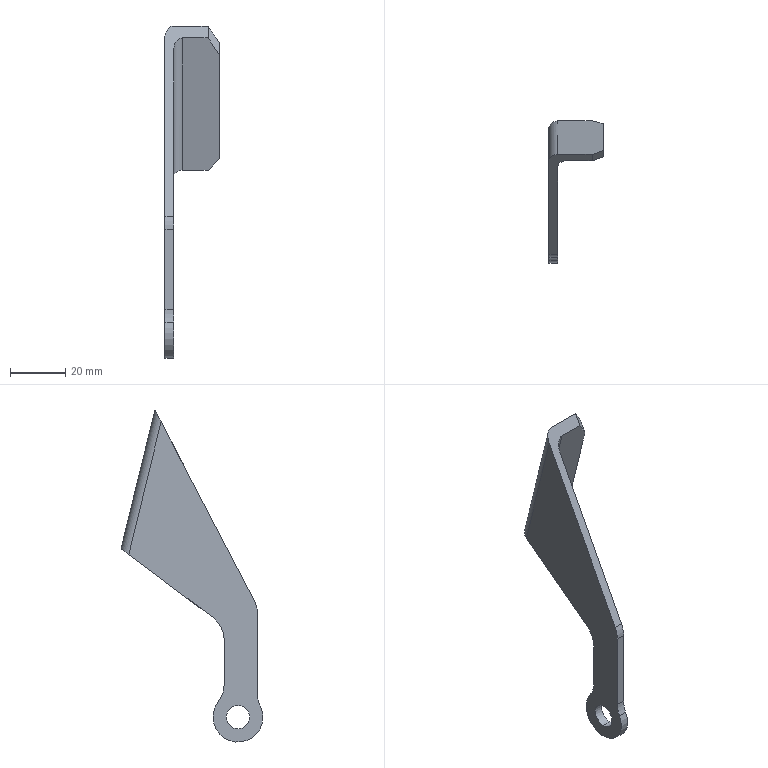Part | SolidWorks | features BaseBody 1 | 1 solid | 20 faces | box 19.6 x 51.2 x 119.9 mm | volume 9604 mm3 | plane 11 | cylinder 9 | commonest cylinder face diameters 20 x4 6.4 x2 8.479 x2 18 x1
STEP:
#1=CARTESIAN_POINT('',(1.6,0.,4.239));
#2=VERTEX_POINT('',#1);
#3=CARTESIAN_POINT('',(1.6,0.,-4.239));
#4=VERTEX_POINT('',#3);
#5=CARTESIAN_POINT('',(1.6,0.,0.));
#6=DIRECTION('',(1.,0.,0.));
#7=DIRECTION('',(0.,0.,1.));
#8=AXIS2_PLACEMENT_3D('',#5,#6,#7);
#9=CIRCLE('',#8,4.239);
#10=EDGE_CURVE('',#2,#4,#9,.T.);
#11=ORIENTED_EDGE('',*,*,#10,.T.);
#12=CARTESIAN_POINT('',(-1.6,0.,-4.239));
#13=VERTEX_POINT('',#12);
#14=CARTESIAN_POINT('',(1.6,0.,-4.239));
#15=DIRECTION('',(-1.,0.,0.));
#16=VECTOR('',#15,1000.);
#17=LINE('',#14,#16);
#18=EDGE_CURVE('',#4,#13,#17,.T.);
#19=ORIENTED_EDGE('',*,*,#18,.T.);
#20=CARTESIAN_POINT('',(-1.6,0.,4.239));
#21=VERTEX_POINT('',#20);
#22=CARTESIAN_POINT('',(-1.6,0.,0.));
#23=DIRECTION('',(-1.,0.,0.));
#24=DIRECTION('',(0.,0.,1.));
#25=AXIS2_PLACEMENT_3D('',#22,#23,#24);
#26=CIRCLE('',#25,4.239);
#27=EDGE_CURVE('',#13,#21,#26,.T.);
#28=ORIENTED_EDGE('',*,*,#27,.T.);
#29=CARTESIAN_POINT('',(1.6,0.,4.239));
#30=DIRECTION('',(-1.,0.,0.));
#31=VECTOR('',#30,1000.);
#32=LINE('',#29,#31);
#33=EDGE_CURVE('',#2,#21,#32,.T.);
#34=ORIENTED_EDGE('',*,*,#33,.F.);
#35=EDGE_LOOP('',(#11,#19,#28,#34));
#36=FACE_OUTER_BOUND('',#35,.T.);
#37=CARTESIAN_POINT('',(1.6,0.,0.));
#38=DIRECTION('',(-1.,0.,0.));
#39=DIRECTION('',(0.,0.,1.));
#40=AXIS2_PLACEMENT_3D('',#37,#38,#39);
#41=CYLINDRICAL_SURFACE('',#40,4.239);
#42=ADVANCED_FACE('',(#36),#41,.F.);
#43=ORIENTED_EDGE('',*,*,#18,.F.);
#44=CARTESIAN_POINT('',(1.6,0.,0.));
#45=DIRECTION('',(1.,0.,0.));
#46=DIRECTION('',(0.,0.,1.));
#47=AXIS2_PLACEMENT_3D('',#44,#45,#46);
#48=CIRCLE('',#47,4.239);
#49=EDGE_CURVE('',#4,#2,#48,.T.);
#50=ORIENTED_EDGE('',*,*,#49,.T.);
#51=ORIENTED_EDGE('',*,*,#33,.T.);
#52=CARTESIAN_POINT('',(-1.6,0.,0.));
#53=DIRECTION('',(-1.,0.,0.));
#54=DIRECTION('',(0.,0.,1.));
#55=AXIS2_PLACEMENT_3D('',#52,#53,#54);
#56=CIRCLE('',#55,4.239);
#57=EDGE_CURVE('',#21,#13,#56,.T.);
#58=ORIENTED_EDGE('',*,*,#57,.T.);
#59=EDGE_LOOP('',(#43,#50,#51,#58));
#60=FACE_OUTER_BOUND('',#59,.T.);
#61=CARTESIAN_POINT('',(1.6,0.,0.));
#62=DIRECTION('',(-1.,0.,0.));
#63=DIRECTION('',(0.,0.,1.));
#64=AXIS2_PLACEMENT_3D('',#61,#62,#63);
#65=CYLINDRICAL_SURFACE('',#64,4.239);
#66=ADVANCED_FACE('',(#60),#65,.F.);
#67=ORIENTED_EDGE('',*,*,#57,.F.);
#68=ORIENTED_EDGE('',*,*,#27,.F.);
#69=EDGE_LOOP('',(#67,#68));
#70=FACE_BOUND('',#69,.T.);
#71=CARTESIAN_POINT('',(-1.6,-7.,8.485));
#72=VERTEX_POINT('',#71);
#73=CARTESIAN_POINT('',(-1.6,-7.,37.451));
#74=VERTEX_POINT('',#73);
#75=CARTESIAN_POINT('',(-1.6,-7.,48.797));
#76=DIRECTION('',(0.,0.,1.));
#77=VECTOR('',#76,1000.);
#78=LINE('',#75,#77);
#79=EDGE_CURVE('',#72,#74,#78,.T.);
#80=ORIENTED_EDGE('',*,*,#79,.T.);
#81=CARTESIAN_POINT('',(-1.6,-5.868,42.072));
#82=VERTEX_POINT('',#81);
#83=CARTESIAN_POINT('',(-1.6,3.,37.451));
#84=DIRECTION('',(-1.,0.,0.));
#85=DIRECTION('',(0.,0.,1.));
#86=AXIS2_PLACEMENT_3D('',#83,#84,#85);
#87=CIRCLE('',#86,10.);
#88=EDGE_CURVE('',#74,#82,#87,.T.);
#89=ORIENTED_EDGE('',*,*,#88,.T.);
#90=CARTESIAN_POINT('',(-1.6,27.757,106.595));
#91=VERTEX_POINT('',#90);
#92=CARTESIAN_POINT('',(-1.6,-5.868,42.072));
#93=DIRECTION('',(0.,0.4621,0.8868));
#94=VECTOR('',#93,1000.);
#95=LINE('',#92,#94);
#96=EDGE_CURVE('',#82,#91,#95,.T.);
#97=ORIENTED_EDGE('',*,*,#96,.T.);
#98=CARTESIAN_POINT('',(-1.6,39.417,58.805));
#99=VERTEX_POINT('',#98);
#100=CARTESIAN_POINT('',(-1.6,27.757,106.595));
#101=DIRECTION('',(0.,0.237,-0.9715));
#102=VECTOR('',#101,1000.);
#103=LINE('',#100,#102);
#104=EDGE_CURVE('',#91,#99,#103,.T.);
#105=ORIENTED_EDGE('',*,*,#104,.T.);
#106=CARTESIAN_POINT('',(-1.6,8.986,35.9));
#107=VERTEX_POINT('',#106);
#108=CARTESIAN_POINT('',(-1.6,39.417,58.805));
#109=DIRECTION('',(0.,-0.799,-0.6014));
#110=VECTOR('',#109,1000.);
#111=LINE('',#108,#110);
#112=EDGE_CURVE('',#99,#107,#111,.T.);
#113=ORIENTED_EDGE('',*,*,#112,.T.);
#114=CARTESIAN_POINT('',(-1.6,5.,27.911));
#115=VERTEX_POINT('',#114);
#116=CARTESIAN_POINT('',(-1.6,15.,27.911));
#117=DIRECTION('',(1.,0.,0.));
#118=DIRECTION('',(0.,0.,1.));
#119=AXIS2_PLACEMENT_3D('',#116,#117,#118);
#120=CIRCLE('',#119,10.);
#121=EDGE_CURVE('',#107,#115,#120,.T.);
#122=ORIENTED_EDGE('',*,*,#121,.T.);
#123=CARTESIAN_POINT('',(-1.6,5.,11.662));
#124=VERTEX_POINT('',#123);
#125=CARTESIAN_POINT('',(-1.6,5.,48.797));
#126=DIRECTION('',(0.,0.,-1.));
#127=VECTOR('',#126,1000.);
#128=LINE('',#125,#127);
#129=EDGE_CURVE('',#115,#124,#128,.T.);
#130=ORIENTED_EDGE('',*,*,#129,.T.);
#131=CARTESIAN_POINT('',(-1.6,7.105,5.524));
#132=VERTEX_POINT('',#131);
#133=CARTESIAN_POINT('',(-1.6,15.,11.662));
#134=DIRECTION('',(1.,0.,0.));
#135=DIRECTION('',(0.,0.,1.));
#136=AXIS2_PLACEMENT_3D('',#133,#134,#135);
#137=CIRCLE('',#136,10.);
#138=EDGE_CURVE('',#124,#132,#137,.T.);
#139=ORIENTED_EDGE('',*,*,#138,.T.);
#140=CARTESIAN_POINT('',(-1.6,-8.053,4.019));
#141=VERTEX_POINT('',#140);
#142=CARTESIAN_POINT('',(-1.6,0.,0.));
#143=DIRECTION('',(-1.,0.,0.));
#144=DIRECTION('',(0.,0.,1.));
#145=AXIS2_PLACEMENT_3D('',#142,#143,#144);
#146=CIRCLE('',#145,9.);
#147=EDGE_CURVE('',#132,#141,#146,.T.);
#148=ORIENTED_EDGE('',*,*,#147,.T.);
#149=CARTESIAN_POINT('',(-1.6,-17.,8.485));
#150=DIRECTION('',(1.,0.,0.));
#151=DIRECTION('',(0.,0.,1.));
#152=AXIS2_PLACEMENT_3D('',#149,#150,#151);
#153=CIRCLE('',#152,10.);
#154=EDGE_CURVE('',#141,#72,#153,.T.);
#155=ORIENTED_EDGE('',*,*,#154,.T.);
#156=EDGE_LOOP('',(#80,#89,#97,#105,#113,#122,#130,#139,#148,#155));
#157=FACE_OUTER_BOUND('',#156,.T.);
#158=CARTESIAN_POINT('',(-1.6,-9.291,-9.694));
#159=DIRECTION('',(-1.,0.,0.));
#160=DIRECTION('',(0.,0.,1.));
#161=AXIS2_PLACEMENT_3D('',#158,#159,#160);
#162=PLANE('',#161);
#163=ADVANCED_FACE('',(#70,#157),#162,.T.);
#164=ORIENTED_EDGE('',*,*,#10,.F.);
#165=ORIENTED_EDGE('',*,*,#49,.F.);
#166=EDGE_LOOP('',(#164,#165));
#167=FACE_BOUND('',#166,.T.);
#168=CARTESIAN_POINT('',(1.6,25.513,102.29));
#169=VERTEX_POINT('',#168);
#170=CARTESIAN_POINT('',(1.6,36.634,56.711));
#171=VERTEX_POINT('',#170);
#172=CARTESIAN_POINT('',(1.6,36.706,56.416));
#173=DIRECTION('',(0.,0.237,-0.9715));
#174=VECTOR('',#173,1000.);
#175=LINE('',#172,#174);
#176=EDGE_CURVE('',#169,#171,#175,.T.);
#177=ORIENTED_EDGE('',*,*,#176,.F.);
#178=CARTESIAN_POINT('',(1.6,-5.868,42.072));
#179=VERTEX_POINT('',#178);
#180=CARTESIAN_POINT('',(1.6,-5.868,42.072));
#181=DIRECTION('',(0.,0.4621,0.8868));
#182=VECTOR('',#181,1000.);
#183=LINE('',#180,#182);
#184=EDGE_CURVE('',#179,#169,#183,.T.);
#185=ORIENTED_EDGE('',*,*,#184,.F.);
#186=CARTESIAN_POINT('',(1.6,-7.,37.451));
#187=VERTEX_POINT('',#186);
#188=CARTESIAN_POINT('',(1.6,3.,37.451));
#189=DIRECTION('',(-1.,0.,0.));
#190=DIRECTION('',(0.,0.,1.));
#191=AXIS2_PLACEMENT_3D('',#188,#189,#190);
#192=CIRCLE('',#191,10.);
#193=EDGE_CURVE('',#187,#179,#192,.T.);
#194=ORIENTED_EDGE('',*,*,#193,.F.);
#195=CARTESIAN_POINT('',(1.6,-7.,8.485));
#196=VERTEX_POINT('',#195);
#197=CARTESIAN_POINT('',(1.6,-7.,46.645));
#198=DIRECTION('',(0.,0.,1.));
#199=VECTOR('',#198,1000.);
#200=LINE('',#197,#199);
#201=EDGE_CURVE('',#196,#187,#200,.T.);
#202=ORIENTED_EDGE('',*,*,#201,.F.);
#203=CARTESIAN_POINT('',(1.6,-8.053,4.019));
#204=VERTEX_POINT('',#203);
#205=CARTESIAN_POINT('',(1.6,-17.,8.485));
#206=DIRECTION('',(1.,0.,0.));
#207=DIRECTION('',(0.,0.,1.));
#208=AXIS2_PLACEMENT_3D('',#205,#206,#207);
#209=CIRCLE('',#208,10.);
#210=EDGE_CURVE('',#204,#196,#209,.T.);
#211=ORIENTED_EDGE('',*,*,#210,.F.);
#212=CARTESIAN_POINT('',(1.6,7.105,5.524));
#213=VERTEX_POINT('',#212);
#214=CARTESIAN_POINT('',(1.6,0.,0.));
#215=DIRECTION('',(-1.,0.,0.));
#216=DIRECTION('',(0.,0.,1.));
#217=AXIS2_PLACEMENT_3D('',#214,#215,#216);
#218=CIRCLE('',#217,9.);
#219=EDGE_CURVE('',#213,#204,#218,.T.);
#220=ORIENTED_EDGE('',*,*,#219,.F.);
#221=CARTESIAN_POINT('',(1.6,5.,11.662));
#222=VERTEX_POINT('',#221);
#223=CARTESIAN_POINT('',(1.6,15.,11.662));
#224=DIRECTION('',(1.,0.,0.));
#225=DIRECTION('',(0.,0.,1.));
#226=AXIS2_PLACEMENT_3D('',#223,#224,#225);
#227=CIRCLE('',#226,10.);
#228=EDGE_CURVE('',#222,#213,#227,.T.);
#229=ORIENTED_EDGE('',*,*,#228,.F.);
#230=CARTESIAN_POINT('',(1.6,5.,27.911));
#231=VERTEX_POINT('',#230);
#232=CARTESIAN_POINT('',(1.6,5.,46.645));
#233=DIRECTION('',(0.,0.,-1.));
#234=VECTOR('',#233,1000.);
#235=LINE('',#232,#234);
#236=EDGE_CURVE('',#231,#222,#235,.T.);
#237=ORIENTED_EDGE('',*,*,#236,.F.);
#238=CARTESIAN_POINT('',(1.6,8.986,35.9));
#239=VERTEX_POINT('',#238);
#240=CARTESIAN_POINT('',(1.6,15.,27.911));
#241=DIRECTION('',(1.,0.,0.));
#242=DIRECTION('',(0.,0.,1.));
#243=AXIS2_PLACEMENT_3D('',#240,#241,#242);
#244=CIRCLE('',#243,10.);
#245=EDGE_CURVE('',#239,#231,#244,.T.);
#246=ORIENTED_EDGE('',*,*,#245,.F.);
#247=CARTESIAN_POINT('',(1.6,42.2,60.9));
#248=DIRECTION('',(0.,-0.799,-0.6014));
#249=VECTOR('',#248,1000.);
#250=LINE('',#247,#249);
#251=EDGE_CURVE('',#171,#239,#250,.T.);
#252=ORIENTED_EDGE('',*,*,#251,.F.);
#253=EDGE_LOOP('',(#177,#185,#194,#202,#211,#220,#229,#237,#246,#252));
#254=FACE_OUTER_BOUND('',#253,.T.);
#255=CARTESIAN_POINT('',(1.6,-9.274,-9.668));
#256=DIRECTION('',(-1.,0.,0.));
#257=DIRECTION('',(0.,0.,1.));
#258=AXIS2_PLACEMENT_3D('',#255,#256,#257);
#259=PLANE('',#258);
#260=ADVANCED_FACE('',(#167,#254),#259,.F.);
#261=CARTESIAN_POINT('',(0.,-7.,37.451));
#262=DIRECTION('',(-1.,0.,0.));
#263=VECTOR('',#262,1000.);
#264=LINE('',#261,#263);
#265=EDGE_CURVE('',#187,#74,#264,.T.);
#266=ORIENTED_EDGE('',*,*,#265,.F.);
#267=ORIENTED_EDGE('',*,*,#193,.T.);
#268=CARTESIAN_POINT('',(0.,-5.868,42.072));
#269=DIRECTION('',(1.,0.,0.));
#270=VECTOR('',#269,1000.);
#271=LINE('',#268,#270);
#272=EDGE_CURVE('',#82,#179,#271,.T.);
#273=ORIENTED_EDGE('',*,*,#272,.F.);
#274=ORIENTED_EDGE('',*,*,#88,.F.);
#275=EDGE_LOOP('',(#266,#267,#273,#274));
#276=FACE_OUTER_BOUND('',#275,.T.);
#277=CARTESIAN_POINT('',(1.6,3.,37.451));
#278=DIRECTION('',(-1.,0.,0.));
#279=DIRECTION('',(0.,0.,1.));
#280=AXIS2_PLACEMENT_3D('',#277,#278,#279);
#281=CYLINDRICAL_SURFACE('',#280,10.);
#282=ADVANCED_FACE('',(#276),#281,.T.);
#283=CARTESIAN_POINT('',(0.,-7.,8.485));
#284=DIRECTION('',(-1.,0.,0.));
#285=VECTOR('',#284,1000.);
#286=LINE('',#283,#285);
#287=EDGE_CURVE('',#196,#72,#286,.T.);
#288=ORIENTED_EDGE('',*,*,#287,.F.);
#289=ORIENTED_EDGE('',*,*,#201,.T.);
#290=ORIENTED_EDGE('',*,*,#265,.T.);
#291=ORIENTED_EDGE('',*,*,#79,.F.);
#292=EDGE_LOOP('',(#288,#289,#290,#291));
#293=FACE_OUTER_BOUND('',#292,.T.);
#294=CARTESIAN_POINT('',(-1.6,-7.,8.485));
#295=DIRECTION('',(0.,1.,0.));
#296=DIRECTION('',(0.,0.,1.));
#297=AXIS2_PLACEMENT_3D('',#294,#295,#296);
#298=PLANE('',#297);
#299=ADVANCED_FACE('',(#293),#298,.F.);
#300=ORIENTED_EDGE('',*,*,#210,.T.);
#301=ORIENTED_EDGE('',*,*,#287,.T.);
#302=ORIENTED_EDGE('',*,*,#154,.F.);
#303=CARTESIAN_POINT('',(0.,-8.053,4.019));
#304=DIRECTION('',(1.,0.,0.));
#305=VECTOR('',#304,1000.);
#306=LINE('',#303,#305);
#307=EDGE_CURVE('',#141,#204,#306,.T.);
#308=ORIENTED_EDGE('',*,*,#307,.T.);
#309=EDGE_LOOP('',(#300,#301,#302,#308));
#310=FACE_OUTER_BOUND('',#309,.T.);
#311=CARTESIAN_POINT('',(1.6,-17.,8.485));
#312=DIRECTION('',(-1.,0.,0.));
#313=DIRECTION('',(0.,0.,1.));
#314=AXIS2_PLACEMENT_3D('',#311,#312,#313);
#315=CYLINDRICAL_SURFACE('',#314,10.);
#316=ADVANCED_FACE('',(#310),#315,.F.);
#317=CARTESIAN_POINT('',(0.,7.105,5.524));
#318=DIRECTION('',(-1.,0.,0.));
#319=VECTOR('',#318,1000.);
#320=LINE('',#317,#319);
#321=EDGE_CURVE('',#213,#132,#320,.T.);
#322=ORIENTED_EDGE('',*,*,#321,.F.);
#323=ORIENTED_EDGE('',*,*,#219,.T.);
#324=ORIENTED_EDGE('',*,*,#307,.F.);
#325=ORIENTED_EDGE('',*,*,#147,.F.);
#326=EDGE_LOOP('',(#322,#323,#324,#325));
#327=FACE_OUTER_BOUND('',#326,.T.);
#328=CARTESIAN_POINT('',(1.6,0.,0.));
#329=DIRECTION('',(-1.,0.,0.));
#330=DIRECTION('',(0.,0.,1.));
#331=AXIS2_PLACEMENT_3D('',#328,#329,#330);
#332=CYLINDRICAL_SURFACE('',#331,9.);
#333=ADVANCED_FACE('',(#327),#332,.T.);
#334=ORIENTED_EDGE('',*,*,#228,.T.);
#335=ORIENTED_EDGE('',*,*,#321,.T.);
#336=ORIENTED_EDGE('',*,*,#138,.F.);
#337=CARTESIAN_POINT('',(0.,5.,11.662));
#338=DIRECTION('',(1.,0.,0.));
#339=VECTOR('',#338,1000.);
#340=LINE('',#337,#339);
#341=EDGE_CURVE('',#124,#222,#340,.T.);
#342=ORIENTED_EDGE('',*,*,#341,.T.);
#343=EDGE_LOOP('',(#334,#335,#336,#342));
#344=FACE_OUTER_BOUND('',#343,.T.);
#345=CARTESIAN_POINT('',(1.6,15.,11.662));
#346=DIRECTION('',(-1.,0.,0.));
#347=DIRECTION('',(0.,0.,1.));
#348=AXIS2_PLACEMENT_3D('',#345,#346,#347);
#349=CYLINDRICAL_SURFACE('',#348,10.);
#350=ADVANCED_FACE('',(#344),#349,.F.);
#351=CARTESIAN_POINT('',(0.,5.,27.911));
#352=DIRECTION('',(-1.,0.,0.));
#353=VECTOR('',#352,1000.);
#354=LINE('',#351,#353);
#355=EDGE_CURVE('',#231,#115,#354,.T.);
#356=ORIENTED_EDGE('',*,*,#355,.F.);
#357=ORIENTED_EDGE('',*,*,#236,.T.);
#358=ORIENTED_EDGE('',*,*,#341,.F.);
#359=ORIENTED_EDGE('',*,*,#129,.F.);
#360=EDGE_LOOP('',(#356,#357,#358,#359));
#361=FACE_OUTER_BOUND('',#360,.T.);
#362=CARTESIAN_POINT('',(-1.6,5.,27.911));
#363=DIRECTION('',(0.,-1.,0.));
#364=DIRECTION('',(0.,0.,-1.));
#365=AXIS2_PLACEMENT_3D('',#362,#363,#364);
#366=PLANE('',#365);
#367=ADVANCED_FACE('',(#361),#366,.F.);
#368=ORIENTED_EDGE('',*,*,#245,.T.);
#369=ORIENTED_EDGE('',*,*,#355,.T.);
#370=ORIENTED_EDGE('',*,*,#121,.F.);
#371=CARTESIAN_POINT('',(0.,8.986,35.9));
#372=DIRECTION('',(1.,0.,0.));
#373=VECTOR('',#372,1000.);
#374=LINE('',#371,#373);
#375=EDGE_CURVE('',#107,#239,#374,.T.);
#376=ORIENTED_EDGE('',*,*,#375,.T.);
#377=EDGE_LOOP('',(#368,#369,#370,#376));
#378=FACE_OUTER_BOUND('',#377,.T.);
#379=CARTESIAN_POINT('',(1.6,15.,27.911));
#380=DIRECTION('',(-1.,0.,0.));
#381=DIRECTION('',(0.,0.,1.));
#382=AXIS2_PLACEMENT_3D('',#379,#380,#381);
#383=CYLINDRICAL_SURFACE('',#382,10.);
#384=ADVANCED_FACE('',(#378),#383,.F.);
#385=CARTESIAN_POINT('',(1.6,42.2,60.9));
#386=VERTEX_POINT('',#385);
#387=CARTESIAN_POINT('',(1.6,42.2,60.9));
#388=CARTESIAN_POINT('',(-0.2745,42.2,60.9));
#389=CARTESIAN_POINT('',(-1.6,41.047,60.032));
#390=CARTESIAN_POINT('',(-1.6,39.417,58.805));
#391=(BOUNDED_CURVE()B_SPLINE_CURVE(3,(#387,#388,#389,#390),.UNSPECIFIED.,.F.,.F.)B_SPLINE_CURVE_WITH_KNOTS((4,4),(3.142,4.712),.UNSPECIFIED.)CURVE()GEOMETRIC_REPRESENTATION_ITEM()RATIONAL_B_SPLINE_CURVE((1.,0.8047,0.8047,1.))REPRESENTATION_ITEM(''));
#392=EDGE_CURVE('',#386,#99,#391,.T.);
#393=ORIENTED_EDGE('',*,*,#392,.F.);
#394=CARTESIAN_POINT('',(14.,42.2,60.9));
#395=VERTEX_POINT('',#394);
#396=CARTESIAN_POINT('',(6.2,42.2,60.9));
#397=DIRECTION('',(-1.,0.,0.));
#398=VECTOR('',#397,1000.);
#399=LINE('',#396,#398);
#400=EDGE_CURVE('',#395,#386,#399,.T.);
#401=ORIENTED_EDGE('',*,*,#400,.F.);
#402=CARTESIAN_POINT('',(14.,39.417,58.805));
#403=VERTEX_POINT('',#402);
#404=CARTESIAN_POINT('',(14.,25.593,48.4));
#405=DIRECTION('',(0.,0.799,0.6014));
#406=VECTOR('',#405,1000.);
#407=LINE('',#404,#406);
#408=EDGE_CURVE('',#403,#395,#407,.T.);
#409=ORIENTED_EDGE('',*,*,#408,.F.);
#410=CARTESIAN_POINT('',(4.8,39.417,58.805));
#411=VERTEX_POINT('',#410);
#412=CARTESIAN_POINT('',(6.2,39.417,58.805));
#413=DIRECTION('',(1.,0.,0.));
#414=VECTOR('',#413,1000.);
#415=LINE('',#412,#414);
#416=EDGE_CURVE('',#411,#403,#415,.T.);
#417=ORIENTED_EDGE('',*,*,#416,.F.);
#418=CARTESIAN_POINT('',(1.6,36.634,56.711));
#419=CARTESIAN_POINT('',(1.6,38.265,57.938));
#420=CARTESIAN_POINT('',(2.925,39.417,58.805));
#421=CARTESIAN_POINT('',(4.8,39.417,58.805));
#422=(BOUNDED_CURVE()B_SPLINE_CURVE(3,(#418,#419,#420,#421),.UNSPECIFIED.,.F.,.F.)B_SPLINE_CURVE_WITH_KNOTS((4,4),(4.712,6.283),.UNSPECIFIED.)CURVE()GEOMETRIC_REPRESENTATION_ITEM()RATIONAL_B_SPLINE_CURVE((1.,0.8047,0.8047,1.))REPRESENTATION_ITEM(''));
#423=EDGE_CURVE('',#171,#411,#422,.T.);
#424=ORIENTED_EDGE('',*,*,#423,.F.);
#425=ORIENTED_EDGE('',*,*,#251,.T.);
#426=ORIENTED_EDGE('',*,*,#375,.F.);
#427=ORIENTED_EDGE('',*,*,#112,.F.);
#428=EDGE_LOOP('',(#393,#401,#409,#417,#424,#425,#426,#427));
#429=FACE_OUTER_BOUND('',#428,.T.);
#430=CARTESIAN_POINT('',(-1.6,42.2,60.9));
#431=DIRECTION('',(0.,-0.6014,0.799));
#432=DIRECTION('',(0.,-0.799,-0.6014));
#433=AXIS2_PLACEMENT_3D('',#430,#431,#432);
#434=PLANE('',#433);
#435=ADVANCED_FACE('',(#429),#434,.F.);
#436=ORIENTED_EDGE('',*,*,#104,.F.);
#437=CARTESIAN_POINT('',(1.6,30.,110.9));
#438=VERTEX_POINT('',#437);
#439=CARTESIAN_POINT('',(1.6,30.,110.9));
#440=CARTESIAN_POINT('',(-0.2745,30.,110.9));
#441=CARTESIAN_POINT('',(-1.6,29.071,109.117));
#442=CARTESIAN_POINT('',(-1.6,27.757,106.595));
#443=(BOUNDED_CURVE()B_SPLINE_CURVE(3,(#439,#440,#441,#442),.UNSPECIFIED.,.F.,.F.)B_SPLINE_CURVE_WITH_KNOTS((4,4),(3.142,4.712),.UNSPECIFIED.)CURVE()GEOMETRIC_REPRESENTATION_ITEM()RATIONAL_B_SPLINE_CURVE((1.,0.8047,0.8047,1.))REPRESENTATION_ITEM(''));
#444=EDGE_CURVE('',#438,#91,#443,.T.);
#445=ORIENTED_EDGE('',*,*,#444,.F.);
#446=CARTESIAN_POINT('',(1.6,36.263,85.232));
#447=DIRECTION('',(0.,-0.237,0.9715));
#448=VECTOR('',#447,1000.);
#449=LINE('',#446,#448);
#450=EDGE_CURVE('',#386,#438,#449,.T.);
#451=ORIENTED_EDGE('',*,*,#450,.F.);
#452=ORIENTED_EDGE('',*,*,#392,.T.);
#453=EDGE_LOOP('',(#436,#445,#451,#452));
#454=FACE_OUTER_BOUND('',#453,.T.);
#455=CARTESIAN_POINT('',(1.6,26.816,110.449));
#456=DIRECTION('',(0.,0.237,-0.9715));
#457=DIRECTION('',(0.,0.9715,0.237));
#458=AXIS2_PLACEMENT_3D('',#455,#456,#457);
#459=CYLINDRICAL_SURFACE('',#458,3.2);
#460=ADVANCED_FACE('',(#454),#459,.T.);
#461=ORIENTED_EDGE('',*,*,#444,.T.);
#462=ORIENTED_EDGE('',*,*,#96,.F.);
#463=ORIENTED_EDGE('',*,*,#272,.T.);
#464=ORIENTED_EDGE('',*,*,#184,.T.);
#465=CARTESIAN_POINT('',(4.8,27.757,106.595));
#466=VERTEX_POINT('',#465);
#467=CARTESIAN_POINT('',(4.8,27.757,106.595));
#468=CARTESIAN_POINT('',(2.925,27.757,106.595));
#469=CARTESIAN_POINT('',(1.6,26.827,104.812));
#470=CARTESIAN_POINT('',(1.6,25.513,102.29));
#471=(BOUNDED_CURVE()B_SPLINE_CURVE(3,(#467,#468,#469,#470),.UNSPECIFIED.,.F.,.F.)B_SPLINE_CURVE_WITH_KNOTS((4,4),(0.,1.571),.UNSPECIFIED.)CURVE()GEOMETRIC_REPRESENTATION_ITEM()RATIONAL_B_SPLINE_CURVE((1.,0.8047,0.8047,1.))REPRESENTATION_ITEM(''));
#472=EDGE_CURVE('',#466,#169,#471,.T.);
#473=ORIENTED_EDGE('',*,*,#472,.F.);
#474=CARTESIAN_POINT('',(14.,27.757,106.595));
#475=VERTEX_POINT('',#474);
#476=CARTESIAN_POINT('',(6.2,27.757,106.595));
#477=DIRECTION('',(-1.,0.,0.));
#478=VECTOR('',#477,1000.);
#479=LINE('',#476,#478);
#480=EDGE_CURVE('',#475,#466,#479,.T.);
#481=ORIENTED_EDGE('',*,*,#480,.F.);
#482=CARTESIAN_POINT('',(14.,30.,110.9));
#483=VERTEX_POINT('',#482);
#484=CARTESIAN_POINT('',(14.,12.066,76.486));
#485=DIRECTION('',(0.,-0.4621,-0.8868));
#486=VECTOR('',#485,1000.);
#487=LINE('',#484,#486);
#488=EDGE_CURVE('',#483,#475,#487,.T.);
#489=ORIENTED_EDGE('',*,*,#488,.F.);
#490=CARTESIAN_POINT('',(6.2,30.,110.9));
#491=DIRECTION('',(1.,0.,0.));
#492=VECTOR('',#491,1000.);
#493=LINE('',#490,#492);
#494=EDGE_CURVE('',#438,#483,#493,.T.);
#495=ORIENTED_EDGE('',*,*,#494,.F.);
#496=EDGE_LOOP('',(#461,#462,#463,#464,#473,#481,#489,#495));
#497=FACE_OUTER_BOUND('',#496,.T.);
#498=CARTESIAN_POINT('',(-1.6,-5.868,42.072));
#499=DIRECTION('',(0.,0.8868,-0.4621));
#500=DIRECTION('',(0.,0.4621,0.8868));
#501=AXIS2_PLACEMENT_3D('',#498,#499,#500);
#502=PLANE('',#501);
#503=ADVANCED_FACE('',(#497),#502,.F.);
#504=ORIENTED_EDGE('',*,*,#472,.T.);
#505=ORIENTED_EDGE('',*,*,#176,.T.);
#506=ORIENTED_EDGE('',*,*,#423,.T.);
#507=CARTESIAN_POINT('',(4.8,33.75,82.032));
#508=DIRECTION('',(0.,-0.237,0.9715));
#509=VECTOR('',#508,1000.);
#510=LINE('',#507,#509);
#511=EDGE_CURVE('',#411,#466,#510,.T.);
#512=ORIENTED_EDGE('',*,*,#511,.T.);
#513=EDGE_LOOP('',(#504,#505,#506,#512));
#514=FACE_OUTER_BOUND('',#513,.T.);
#515=CARTESIAN_POINT('',(4.8,36.706,56.416));
#516=DIRECTION('',(0.,-0.237,0.9715));
#517=DIRECTION('',(0.,-0.9715,-0.237));
#518=AXIS2_PLACEMENT_3D('',#515,#516,#517);
#519=CYLINDRICAL_SURFACE('',#518,3.2);
#520=ADVANCED_FACE('',(#514),#519,.F.);
#521=ORIENTED_EDGE('',*,*,#450,.T.);
#522=ORIENTED_EDGE('',*,*,#494,.T.);
#523=CARTESIAN_POINT('',(18.,31.438,105.005));
#524=VERTEX_POINT('',#523);
#525=CARTESIAN_POINT('',(18.,31.438,105.005));
#526=DIRECTION('',(-0.5504,-0.1979,0.8111));
#527=VECTOR('',#526,1000.);
#528=LINE('',#525,#527);
#529=EDGE_CURVE('',#524,#483,#528,.T.);
#530=ORIENTED_EDGE('',*,*,#529,.F.);
#531=CARTESIAN_POINT('',(18.,41.168,65.13));
#532=VERTEX_POINT('',#531);
#533=CARTESIAN_POINT('',(18.,36.1,85.9));
#534=DIRECTION('',(0.,-0.237,0.9715));
#535=VECTOR('',#534,1000.);
#536=LINE('',#533,#535);
#537=EDGE_CURVE('',#532,#524,#536,.T.);
#538=ORIENTED_EDGE('',*,*,#537,.F.);
#539=CARTESIAN_POINT('',(14.,42.2,60.9));
#540=DIRECTION('',(0.6766,-0.1746,0.7154));
#541=VECTOR('',#540,1000.);
#542=LINE('',#539,#541);
#543=EDGE_CURVE('',#395,#532,#542,.T.);
#544=ORIENTED_EDGE('',*,*,#543,.F.);
#545=ORIENTED_EDGE('',*,*,#400,.T.);
#546=EDGE_LOOP('',(#521,#522,#530,#538,#544,#545));
#547=FACE_OUTER_BOUND('',#546,.T.);
#548=CARTESIAN_POINT('',(1.6,30.,110.9));
#549=DIRECTION('',(0.,-0.9715,-0.237));
#550=DIRECTION('',(0.,0.237,-0.9715));
#551=AXIS2_PLACEMENT_3D('',#548,#549,#550);
#552=PLANE('',#551);
#553=ADVANCED_FACE('',(#547),#552,.F.);
#554=CARTESIAN_POINT('',(18.,38.385,63.035));
#555=VERTEX_POINT('',#554);
#556=CARTESIAN_POINT('',(18.,38.385,63.035));
#557=DIRECTION('',(-0.6766,0.1746,-0.7154));
#558=VECTOR('',#557,1000.);
#559=LINE('',#556,#558);
#560=EDGE_CURVE('',#555,#403,#559,.T.);
#561=ORIENTED_EDGE('',*,*,#560,.T.);
#562=ORIENTED_EDGE('',*,*,#408,.T.);
#563=ORIENTED_EDGE('',*,*,#543,.T.);
#564=CARTESIAN_POINT('',(18.,41.168,65.13));
#565=DIRECTION('',(0.000000001,-0.799,-0.6014));
#566=VECTOR('',#565,1000.);
#567=LINE('',#564,#566);
#568=EDGE_CURVE('',#532,#555,#567,.T.);
#569=ORIENTED_EDGE('',*,*,#568,.T.);
#570=EDGE_LOOP('',(#561,#562,#563,#569));
#571=FACE_OUTER_BOUND('',#570,.T.);
#572=CARTESIAN_POINT('',(19.058,38.362,64.342));
#573=DIRECTION('',(0.7071,0.4252,-0.565));
#574=DIRECTION('',(-0.6242,0.,-0.7813));
#575=AXIS2_PLACEMENT_3D('',#572,#573,#574);
#576=PLANE('',#575);
#577=ADVANCED_FACE('',(#571),#576,.T.);
#578=CARTESIAN_POINT('',(18.,29.195,100.7));
#579=VERTEX_POINT('',#578);
#580=CARTESIAN_POINT('',(18.,33.587,82.7));
#581=DIRECTION('',(0.,-0.237,0.9715));
#582=VECTOR('',#581,1000.);
#583=LINE('',#580,#582);
#584=EDGE_CURVE('',#555,#579,#583,.T.);
#585=ORIENTED_EDGE('',*,*,#584,.T.);
#586=CARTESIAN_POINT('',(18.,29.195,100.7));
#587=DIRECTION('',(-0.5504,-0.1979,0.8111));
#588=VECTOR('',#587,1000.);
#589=LINE('',#586,#588);
#590=EDGE_CURVE('',#579,#475,#589,.T.);
#591=ORIENTED_EDGE('',*,*,#590,.T.);
#592=ORIENTED_EDGE('',*,*,#480,.T.);
#593=ORIENTED_EDGE('',*,*,#511,.F.);
#594=ORIENTED_EDGE('',*,*,#416,.T.);
#595=ORIENTED_EDGE('',*,*,#560,.F.);
#596=EDGE_LOOP('',(#585,#591,#592,#593,#594,#595));
#597=FACE_OUTER_BOUND('',#596,.T.);
#598=CARTESIAN_POINT('',(4.8,27.757,106.595));
#599=DIRECTION('',(0.,-0.9715,-0.237));
#600=DIRECTION('',(0.,0.237,-0.9715));
#601=AXIS2_PLACEMENT_3D('',#598,#599,#600);
#602=PLANE('',#601);
#603=ADVANCED_FACE('',(#597),#602,.T.);
#604=ORIENTED_EDGE('',*,*,#529,.T.);
#605=ORIENTED_EDGE('',*,*,#488,.T.);
#606=ORIENTED_EDGE('',*,*,#590,.F.);
#607=CARTESIAN_POINT('',(18.,29.195,100.7));
#608=DIRECTION('',(0.,0.4621,0.8868));
#609=VECTOR('',#608,1000.);
#610=LINE('',#607,#609);
#611=EDGE_CURVE('',#579,#524,#610,.T.);
#612=ORIENTED_EDGE('',*,*,#611,.T.);
#613=EDGE_LOOP('',(#604,#605,#606,#612));
#614=FACE_OUTER_BOUND('',#613,.T.);
#615=CARTESIAN_POINT('',(15.519,26.366,100.639));
#616=DIRECTION('',(0.7071,-0.6271,0.3268));
#617=DIRECTION('',(0.6635,0.7482,0.));
#618=AXIS2_PLACEMENT_3D('',#615,#616,#617);
#619=PLANE('',#618);
#620=ADVANCED_FACE('',(#614),#619,.T.);
#621=ORIENTED_EDGE('',*,*,#537,.T.);
#622=ORIENTED_EDGE('',*,*,#611,.F.);
#623=ORIENTED_EDGE('',*,*,#584,.F.);
#624=ORIENTED_EDGE('',*,*,#568,.F.);
#625=EDGE_LOOP('',(#621,#622,#623,#624));
#626=FACE_OUTER_BOUND('',#625,.T.);
#627=CARTESIAN_POINT('',(18.,29.123,105.257));
#628=DIRECTION('',(1.,0.,0.));
#629=DIRECTION('',(0.,0.,-1.));
#630=AXIS2_PLACEMENT_3D('',#627,#628,#629);
#631=PLANE('',#630);
#632=ADVANCED_FACE('',(#626),#631,.T.);
#633=CLOSED_SHELL('',(#42,#66,#163,#260,#282,#299,#316,#333,#350,#367,#384,#435,#460,#503,#520,#553,#577,#603,#620,#632));
#634=MANIFOLD_SOLID_BREP('',#633);
#635=CARTESIAN_POINT('',(0.,0.,0.));
#636=DIRECTION('',(0.,0.,1.));
#637=DIRECTION('',(1.,0.,0.));
#638=AXIS2_PLACEMENT_3D('',#635,#636,#637);
#639=(LENGTH_UNIT()NAMED_UNIT(*)SI_UNIT(.MILLI.,.METRE.));
#640=UNCERTAINTY_MEASURE_WITH_UNIT(LENGTH_MEASURE(0.00001),#639,'','');
#641=(NAMED_UNIT(*)PLANE_ANGLE_UNIT()SI_UNIT($,.RADIAN.));
#642=(NAMED_UNIT(*)SI_UNIT($,.STERADIAN.)SOLID_ANGLE_UNIT());
#643=(GEOMETRIC_REPRESENTATION_CONTEXT(3)GLOBAL_UNCERTAINTY_ASSIGNED_CONTEXT((#640))GLOBAL_UNIT_ASSIGNED_CONTEXT((#639,#641,#642))REPRESENTATION_CONTEXT('',''));
#644=ADVANCED_BREP_SHAPE_REPRESENTATION('',(#634,#638),#643);